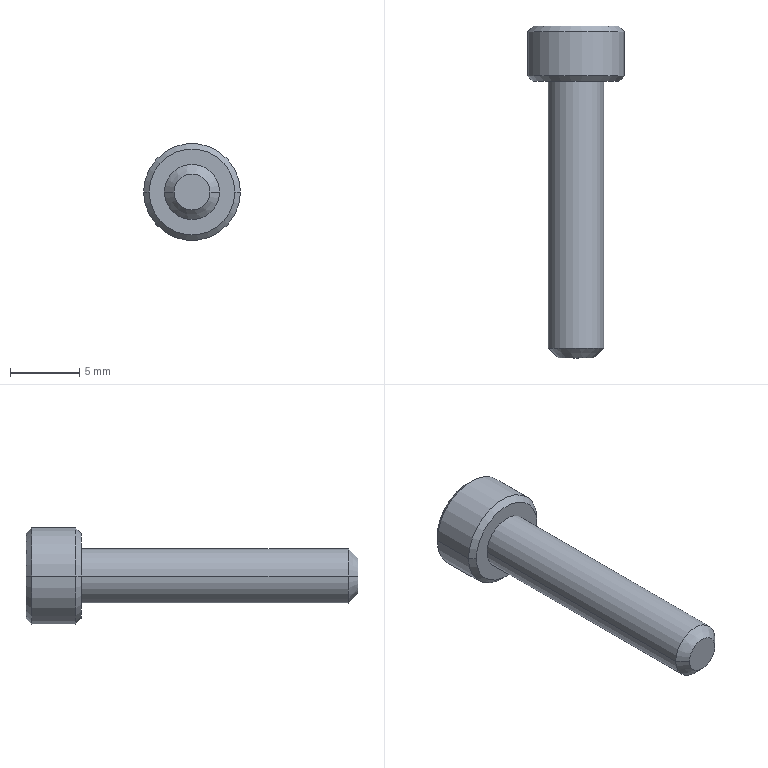Part | STEP file | BB62-M4-20L-3 | 1 solid | 27 faces | box 7 x 24 x 7 mm | volume 380.713 mm3 | plane 15 | cone 8 | cylinder 4 | commonest cylinder face diameters 4 x2 7 x2
STEP:
#1=CARTESIAN_POINT('',(0.,1.007,0.));
#2=VERTEX_POINT('',#1);
#3=CARTESIAN_POINT('',(1.72,2.,0.));
#4=VERTEX_POINT('',#3);
#5=CARTESIAN_POINT('',(0.,1.007,0.));
#6=DIRECTION('',(0.866,0.5,0.));
#7=VECTOR('',#6,1000.);
#8=LINE('',#5,#7);
#9=EDGE_CURVE('',#2,#4,#8,.T.);
#10=ORIENTED_EDGE('',*,*,#9,.F.);
#11=CARTESIAN_POINT('',(-1.72,2.,0.));
#12=VERTEX_POINT('',#11);
#13=CARTESIAN_POINT('',(0.,1.007,0.));
#14=DIRECTION('',(-0.866,0.5,0.));
#15=VECTOR('',#14,1000.);
#16=LINE('',#13,#15);
#17=EDGE_CURVE('',#2,#12,#16,.T.);
#18=ORIENTED_EDGE('',*,*,#17,.T.);
#19=CARTESIAN_POINT('',(-1.49,2.,0.86));
#20=VERTEX_POINT('',#19);
#21=CARTESIAN_POINT('',(0.,2.,0.));
#22=DIRECTION('',(0.,-1.,0.));
#23=DIRECTION('',(-1.,0.,0.));
#24=AXIS2_PLACEMENT_3D('',#21,#22,#23);
#25=CIRCLE('',#24,1.72);
#26=EDGE_CURVE('',#20,#12,#25,.T.);
#27=ORIENTED_EDGE('',*,*,#26,.F.);
#28=CARTESIAN_POINT('',(0.,2.,1.72));
#29=VERTEX_POINT('',#28);
#30=CARTESIAN_POINT('',(0.,2.,0.));
#31=DIRECTION('',(0.,-1.,0.));
#32=DIRECTION('',(-1.,0.,0.));
#33=AXIS2_PLACEMENT_3D('',#30,#31,#32);
#34=CIRCLE('',#33,1.72);
#35=EDGE_CURVE('',#29,#20,#34,.T.);
#36=ORIENTED_EDGE('',*,*,#35,.F.);
#37=CARTESIAN_POINT('',(1.49,2.,0.86));
#38=VERTEX_POINT('',#37);
#39=CARTESIAN_POINT('',(0.,2.,0.));
#40=DIRECTION('',(0.,-1.,0.));
#41=DIRECTION('',(-1.,0.,0.));
#42=AXIS2_PLACEMENT_3D('',#39,#40,#41);
#43=CIRCLE('',#42,1.72);
#44=EDGE_CURVE('',#38,#29,#43,.T.);
#45=ORIENTED_EDGE('',*,*,#44,.F.);
#46=CARTESIAN_POINT('',(0.,2.,0.));
#47=DIRECTION('',(0.,-1.,0.));
#48=DIRECTION('',(-1.,0.,0.));
#49=AXIS2_PLACEMENT_3D('',#46,#47,#48);
#50=CIRCLE('',#49,1.72);
#51=EDGE_CURVE('',#4,#38,#50,.T.);
#52=ORIENTED_EDGE('',*,*,#51,.F.);
#53=EDGE_LOOP('',(#10,#18,#27,#36,#45,#52));
#54=FACE_OUTER_BOUND('',#53,.T.);
#55=CARTESIAN_POINT('',(0.,1001.007,0.));
#56=DIRECTION('',(0.,1.,0.));
#57=DIRECTION('',(1.,0.,0.));
#58=AXIS2_PLACEMENT_3D('',#55,#56,#57);
#59=CONICAL_SURFACE('',#58,1732.051,1.047);
#60=ADVANCED_FACE('',(#54),#59,.F.);
#61=CARTESIAN_POINT('',(1.3,-20.,0.));
#62=VERTEX_POINT('',#61);
#63=CARTESIAN_POINT('',(-1.3,-20.,0.));
#64=VERTEX_POINT('',#63);
#65=CARTESIAN_POINT('',(0.,-20.,0.));
#66=DIRECTION('',(0.,1.,0.));
#67=DIRECTION('',(1.,0.,0.));
#68=AXIS2_PLACEMENT_3D('',#65,#66,#67);
#69=CIRCLE('',#68,1.3);
#70=EDGE_CURVE('',#62,#64,#69,.T.);
#71=ORIENTED_EDGE('',*,*,#70,.T.);
#72=CARTESIAN_POINT('',(-2.,-19.3,0.));
#73=VERTEX_POINT('',#72);
#74=CARTESIAN_POINT('',(-1.3,-20.,0.));
#75=DIRECTION('',(-0.7071,0.7071,0.));
#76=VECTOR('',#75,1000.);
#77=LINE('',#74,#76);
#78=EDGE_CURVE('',#64,#73,#77,.T.);
#79=ORIENTED_EDGE('',*,*,#78,.T.);
#80=CARTESIAN_POINT('',(2.,-19.3,0.));
#81=VERTEX_POINT('',#80);
#82=CARTESIAN_POINT('',(0.,-19.3,0.));
#83=DIRECTION('',(0.,-1.,0.));
#84=DIRECTION('',(-1.,0.,0.));
#85=AXIS2_PLACEMENT_3D('',#82,#83,#84);
#86=CIRCLE('',#85,2.);
#87=EDGE_CURVE('',#73,#81,#86,.T.);
#88=ORIENTED_EDGE('',*,*,#87,.T.);
#89=CARTESIAN_POINT('',(1.3,-20.,0.));
#90=DIRECTION('',(0.7071,0.7071,0.));
#91=VECTOR('',#90,1000.);
#92=LINE('',#89,#91);
#93=EDGE_CURVE('',#62,#81,#92,.T.);
#94=ORIENTED_EDGE('',*,*,#93,.F.);
#95=EDGE_LOOP('',(#71,#79,#88,#94));
#96=FACE_OUTER_BOUND('',#95,.T.);
#97=CARTESIAN_POINT('',(0.,-20.,0.));
#98=DIRECTION('',(0.,1.,0.));
#99=DIRECTION('',(1.,0.,0.));
#100=AXIS2_PLACEMENT_3D('',#97,#98,#99);
#101=CONICAL_SURFACE('',#100,1.3,0.7854);
#102=ADVANCED_FACE('',(#96),#101,.T.);
#103=ORIENTED_EDGE('',*,*,#87,.F.);
#104=CARTESIAN_POINT('',(-2.,0.,0.));
#105=VERTEX_POINT('',#104);
#106=CARTESIAN_POINT('',(-2.,-19.3,0.));
#107=DIRECTION('',(0.,1.,0.));
#108=VECTOR('',#107,1000.);
#109=LINE('',#106,#108);
#110=EDGE_CURVE('',#73,#105,#109,.T.);
#111=ORIENTED_EDGE('',*,*,#110,.T.);
#112=CARTESIAN_POINT('',(2.,0.,0.));
#113=VERTEX_POINT('',#112);
#114=CARTESIAN_POINT('',(0.,0.,0.));
#115=DIRECTION('',(0.,-1.,0.));
#116=DIRECTION('',(-1.,0.,0.));
#117=AXIS2_PLACEMENT_3D('',#114,#115,#116);
#118=CIRCLE('',#117,2.);
#119=EDGE_CURVE('',#105,#113,#118,.T.);
#120=ORIENTED_EDGE('',*,*,#119,.T.);
#121=CARTESIAN_POINT('',(2.,-19.3,0.));
#122=DIRECTION('',(0.,1.,0.));
#123=VECTOR('',#122,1000.);
#124=LINE('',#121,#123);
#125=EDGE_CURVE('',#81,#113,#124,.T.);
#126=ORIENTED_EDGE('',*,*,#125,.F.);
#127=EDGE_LOOP('',(#103,#111,#120,#126));
#128=FACE_OUTER_BOUND('',#127,.T.);
#129=CARTESIAN_POINT('',(0.,-19.3,0.));
#130=DIRECTION('',(0.,1.,0.));
#131=DIRECTION('',(1.,0.,0.));
#132=AXIS2_PLACEMENT_3D('',#129,#130,#131);
#133=CYLINDRICAL_SURFACE('',#132,2.);
#134=ADVANCED_FACE('',(#128),#133,.T.);
#135=CARTESIAN_POINT('',(-3.1,4.,0.));
#136=VERTEX_POINT('',#135);
#137=CARTESIAN_POINT('',(3.1,4.,0.));
#138=VERTEX_POINT('',#137);
#139=CARTESIAN_POINT('',(0.,4.,0.));
#140=DIRECTION('',(0.,-1.,0.));
#141=DIRECTION('',(-1.,0.,0.));
#142=AXIS2_PLACEMENT_3D('',#139,#140,#141);
#143=CIRCLE('',#142,3.1);
#144=EDGE_CURVE('',#136,#138,#143,.T.);
#145=ORIENTED_EDGE('',*,*,#144,.T.);
#146=CARTESIAN_POINT('',(3.5,3.6,0.));
#147=VERTEX_POINT('',#146);
#148=CARTESIAN_POINT('',(3.5,3.6,0.));
#149=DIRECTION('',(0.7071,-0.7071,0.));
#150=VECTOR('',#149,1000.);
#151=LINE('',#148,#150);
#152=EDGE_CURVE('',#138,#147,#151,.T.);
#153=ORIENTED_EDGE('',*,*,#152,.T.);
#154=CARTESIAN_POINT('',(-3.5,3.6,0.));
#155=VERTEX_POINT('',#154);
#156=CARTESIAN_POINT('',(0.,3.6,0.));
#157=DIRECTION('',(0.,-1.,0.));
#158=DIRECTION('',(-1.,0.,0.));
#159=AXIS2_PLACEMENT_3D('',#156,#157,#158);
#160=CIRCLE('',#159,3.5);
#161=EDGE_CURVE('',#155,#147,#160,.T.);
#162=ORIENTED_EDGE('',*,*,#161,.F.);
#163=CARTESIAN_POINT('',(-3.5,3.6,0.));
#164=DIRECTION('',(-0.7071,-0.7071,0.));
#165=VECTOR('',#164,1000.);
#166=LINE('',#163,#165);
#167=EDGE_CURVE('',#136,#155,#166,.T.);
#168=ORIENTED_EDGE('',*,*,#167,.F.);
#169=EDGE_LOOP('',(#145,#153,#162,#168));
#170=FACE_OUTER_BOUND('',#169,.T.);
#171=CARTESIAN_POINT('',(0.,3.6,0.));
#172=DIRECTION('',(0.,-1.,0.));
#173=DIRECTION('',(-1.,0.,0.));
#174=AXIS2_PLACEMENT_3D('',#171,#172,#173);
#175=CONICAL_SURFACE('',#174,3.5,0.7854);
#176=ADVANCED_FACE('',(#170),#175,.T.);
#177=ORIENTED_EDGE('',*,*,#161,.T.);
#178=CARTESIAN_POINT('',(3.5,0.4,0.));
#179=VERTEX_POINT('',#178);
#180=CARTESIAN_POINT('',(3.5,1.62,0.));
#181=DIRECTION('',(0.,-1.,0.));
#182=VECTOR('',#181,1000.);
#183=LINE('',#180,#182);
#184=EDGE_CURVE('',#147,#179,#183,.T.);
#185=ORIENTED_EDGE('',*,*,#184,.T.);
#186=CARTESIAN_POINT('',(-3.5,0.4,0.));
#187=VERTEX_POINT('',#186);
#188=CARTESIAN_POINT('',(0.,0.4,0.));
#189=DIRECTION('',(0.,-1.,0.));
#190=DIRECTION('',(-1.,0.,0.));
#191=AXIS2_PLACEMENT_3D('',#188,#189,#190);
#192=CIRCLE('',#191,3.5);
#193=EDGE_CURVE('',#187,#179,#192,.T.);
#194=ORIENTED_EDGE('',*,*,#193,.F.);
#195=CARTESIAN_POINT('',(-3.5,1.62,0.));
#196=DIRECTION('',(0.,-1.,0.));
#197=VECTOR('',#196,1000.);
#198=LINE('',#195,#197);
#199=EDGE_CURVE('',#155,#187,#198,.T.);
#200=ORIENTED_EDGE('',*,*,#199,.F.);
#201=EDGE_LOOP('',(#177,#185,#194,#200));
#202=FACE_OUTER_BOUND('',#201,.T.);
#203=CARTESIAN_POINT('',(0.,1.62,0.));
#204=DIRECTION('',(0.,-1.,0.));
#205=DIRECTION('',(-1.,0.,0.));
#206=AXIS2_PLACEMENT_3D('',#203,#204,#205);
#207=CYLINDRICAL_SURFACE('',#206,3.5);
#208=ADVANCED_FACE('',(#202),#207,.T.);
#209=CARTESIAN_POINT('',(-3.1,0.,0.));
#210=VERTEX_POINT('',#209);
#211=CARTESIAN_POINT('',(3.1,0.,0.));
#212=VERTEX_POINT('',#211);
#213=CARTESIAN_POINT('',(0.,0.,0.));
#214=DIRECTION('',(0.,-1.,0.));
#215=DIRECTION('',(-1.,0.,0.));
#216=AXIS2_PLACEMENT_3D('',#213,#214,#215);
#217=CIRCLE('',#216,3.1);
#218=EDGE_CURVE('',#210,#212,#217,.T.);
#219=ORIENTED_EDGE('',*,*,#218,.F.);
#220=CARTESIAN_POINT('',(-3.1,0.,0.));
#221=DIRECTION('',(-0.7071,0.7071,0.));
#222=VECTOR('',#221,1000.);
#223=LINE('',#220,#222);
#224=EDGE_CURVE('',#210,#187,#223,.T.);
#225=ORIENTED_EDGE('',*,*,#224,.T.);
#226=ORIENTED_EDGE('',*,*,#193,.T.);
#227=CARTESIAN_POINT('',(3.1,0.,0.));
#228=DIRECTION('',(0.7071,0.7071,0.));
#229=VECTOR('',#228,1000.);
#230=LINE('',#227,#229);
#231=EDGE_CURVE('',#212,#179,#230,.T.);
#232=ORIENTED_EDGE('',*,*,#231,.F.);
#233=EDGE_LOOP('',(#219,#225,#226,#232));
#234=FACE_OUTER_BOUND('',#233,.T.);
#235=CARTESIAN_POINT('',(0.,0.,0.));
#236=DIRECTION('',(0.,1.,0.));
#237=DIRECTION('',(1.,0.,0.));
#238=AXIS2_PLACEMENT_3D('',#235,#236,#237);
#239=CONICAL_SURFACE('',#238,3.1,0.7854);
#240=ADVANCED_FACE('',(#234),#239,.T.);
#241=ORIENTED_EDGE('',*,*,#144,.F.);
#242=CARTESIAN_POINT('',(0.,4.,0.));
#243=DIRECTION('',(0.,-1.,0.));
#244=DIRECTION('',(-1.,0.,0.));
#245=AXIS2_PLACEMENT_3D('',#242,#243,#244);
#246=CIRCLE('',#245,3.1);
#247=EDGE_CURVE('',#138,#136,#246,.T.);
#248=ORIENTED_EDGE('',*,*,#247,.F.);
#249=EDGE_LOOP('',(#241,#248));
#250=FACE_OUTER_BOUND('',#249,.T.);
#251=CARTESIAN_POINT('',(0.,4.,-1.72));
#252=VERTEX_POINT('',#251);
#253=CARTESIAN_POINT('',(-1.49,4.,-0.86));
#254=VERTEX_POINT('',#253);
#255=CARTESIAN_POINT('',(0.,4.,-1.72));
#256=DIRECTION('',(-0.866,0.,0.5));
#257=VECTOR('',#256,1000.);
#258=LINE('',#255,#257);
#259=EDGE_CURVE('',#252,#254,#258,.T.);
#260=ORIENTED_EDGE('',*,*,#259,.F.);
#261=CARTESIAN_POINT('',(1.49,4.,-0.86));
#262=VERTEX_POINT('',#261);
#263=CARTESIAN_POINT('',(1.49,4.,-0.86));
#264=DIRECTION('',(-0.866,0.,-0.5));
#265=VECTOR('',#264,1000.);
#266=LINE('',#263,#265);
#267=EDGE_CURVE('',#262,#252,#266,.T.);
#268=ORIENTED_EDGE('',*,*,#267,.F.);
#269=CARTESIAN_POINT('',(1.49,4.,0.86));
#270=VERTEX_POINT('',#269);
#271=CARTESIAN_POINT('',(1.49,4.,0.86));
#272=DIRECTION('',(0.,0.,-1.));
#273=VECTOR('',#272,1000.);
#274=LINE('',#271,#273);
#275=EDGE_CURVE('',#270,#262,#274,.T.);
#276=ORIENTED_EDGE('',*,*,#275,.F.);
#277=CARTESIAN_POINT('',(0.,4.,1.72));
#278=VERTEX_POINT('',#277);
#279=CARTESIAN_POINT('',(0.,4.,1.72));
#280=DIRECTION('',(0.866,0.,-0.5));
#281=VECTOR('',#280,1000.);
#282=LINE('',#279,#281);
#283=EDGE_CURVE('',#278,#270,#282,.T.);
#284=ORIENTED_EDGE('',*,*,#283,.F.);
#285=CARTESIAN_POINT('',(-1.49,4.,0.86));
#286=VERTEX_POINT('',#285);
#287=CARTESIAN_POINT('',(-1.49,4.,0.86));
#288=DIRECTION('',(0.866,0.,0.5));
#289=VECTOR('',#288,1000.);
#290=LINE('',#287,#289);
#291=EDGE_CURVE('',#286,#278,#290,.T.);
#292=ORIENTED_EDGE('',*,*,#291,.F.);
#293=CARTESIAN_POINT('',(-1.49,4.,-0.86));
#294=DIRECTION('',(0.,0.,1.));
#295=VECTOR('',#294,1000.);
#296=LINE('',#293,#295);
#297=EDGE_CURVE('',#254,#286,#296,.T.);
#298=ORIENTED_EDGE('',*,*,#297,.F.);
#299=EDGE_LOOP('',(#260,#268,#276,#284,#292,#298));
#300=FACE_BOUND('',#299,.T.);
#301=CARTESIAN_POINT('',(3.1,4.,0.));
#302=DIRECTION('',(0.,1.,0.));
#303=DIRECTION('',(1.,0.,0.));
#304=AXIS2_PLACEMENT_3D('',#301,#302,#303);
#305=PLANE('',#304);
#306=ADVANCED_FACE('',(#250,#300),#305,.T.);
#307=CARTESIAN_POINT('',(0.,0.,0.));
#308=DIRECTION('',(0.,-1.,0.));
#309=DIRECTION('',(-1.,0.,0.));
#310=AXIS2_PLACEMENT_3D('',#307,#308,#309);
#311=CIRCLE('',#310,2.);
#312=EDGE_CURVE('',#113,#105,#311,.T.);
#313=ORIENTED_EDGE('',*,*,#312,.F.);
#314=ORIENTED_EDGE('',*,*,#119,.F.);
#315=EDGE_LOOP('',(#313,#314));
#316=FACE_BOUND('',#315,.T.);
#317=CARTESIAN_POINT('',(0.,0.,0.));
#318=DIRECTION('',(0.,-1.,0.));
#319=DIRECTION('',(-1.,0.,0.));
#320=AXIS2_PLACEMENT_3D('',#317,#318,#319);
#321=CIRCLE('',#320,3.1);
#322=EDGE_CURVE('',#212,#210,#321,.T.);
#323=ORIENTED_EDGE('',*,*,#322,.T.);
#324=ORIENTED_EDGE('',*,*,#218,.T.);
#325=EDGE_LOOP('',(#323,#324));
#326=FACE_OUTER_BOUND('',#325,.T.);
#327=CARTESIAN_POINT('',(0.,0.,0.));
#328=DIRECTION('',(0.,-1.,0.));
#329=DIRECTION('',(-1.,0.,0.));
#330=AXIS2_PLACEMENT_3D('',#327,#328,#329);
#331=PLANE('',#330);
#332=ADVANCED_FACE('',(#316,#326),#331,.T.);
#333=ORIENTED_EDGE('',*,*,#224,.F.);
#334=ORIENTED_EDGE('',*,*,#322,.F.);
#335=ORIENTED_EDGE('',*,*,#231,.T.);
#336=CARTESIAN_POINT('',(0.,0.4,0.));
#337=DIRECTION('',(0.,-1.,0.));
#338=DIRECTION('',(-1.,0.,0.));
#339=AXIS2_PLACEMENT_3D('',#336,#337,#338);
#340=CIRCLE('',#339,3.5);
#341=EDGE_CURVE('',#179,#187,#340,.T.);
#342=ORIENTED_EDGE('',*,*,#341,.T.);
#343=EDGE_LOOP('',(#333,#334,#335,#342));
#344=FACE_OUTER_BOUND('',#343,.T.);
#345=CARTESIAN_POINT('',(0.,0.,0.));
#346=DIRECTION('',(0.,1.,0.));
#347=DIRECTION('',(1.,0.,0.));
#348=AXIS2_PLACEMENT_3D('',#345,#346,#347);
#349=CONICAL_SURFACE('',#348,3.1,0.7854);
#350=ADVANCED_FACE('',(#344),#349,.T.);
#351=ORIENTED_EDGE('',*,*,#184,.F.);
#352=CARTESIAN_POINT('',(0.,3.6,0.));
#353=DIRECTION('',(0.,-1.,0.));
#354=DIRECTION('',(-1.,0.,0.));
#355=AXIS2_PLACEMENT_3D('',#352,#353,#354);
#356=CIRCLE('',#355,3.5);
#357=EDGE_CURVE('',#147,#155,#356,.T.);
#358=ORIENTED_EDGE('',*,*,#357,.T.);
#359=ORIENTED_EDGE('',*,*,#199,.T.);
#360=ORIENTED_EDGE('',*,*,#341,.F.);
#361=EDGE_LOOP('',(#351,#358,#359,#360));
#362=FACE_OUTER_BOUND('',#361,.T.);
#363=CARTESIAN_POINT('',(0.,1.62,0.));
#364=DIRECTION('',(0.,-1.,0.));
#365=DIRECTION('',(-1.,0.,0.));
#366=AXIS2_PLACEMENT_3D('',#363,#364,#365);
#367=CYLINDRICAL_SURFACE('',#366,3.5);
#368=ADVANCED_FACE('',(#362),#367,.T.);
#369=ORIENTED_EDGE('',*,*,#152,.F.);
#370=ORIENTED_EDGE('',*,*,#247,.T.);
#371=ORIENTED_EDGE('',*,*,#167,.T.);
#372=ORIENTED_EDGE('',*,*,#357,.F.);
#373=EDGE_LOOP('',(#369,#370,#371,#372));
#374=FACE_OUTER_BOUND('',#373,.T.);
#375=CARTESIAN_POINT('',(0.,3.6,0.));
#376=DIRECTION('',(0.,-1.,0.));
#377=DIRECTION('',(-1.,0.,0.));
#378=AXIS2_PLACEMENT_3D('',#375,#376,#377);
#379=CONICAL_SURFACE('',#378,3.5,0.7854);
#380=ADVANCED_FACE('',(#374),#379,.T.);
#381=ORIENTED_EDGE('',*,*,#110,.F.);
#382=CARTESIAN_POINT('',(0.,-19.3,0.));
#383=DIRECTION('',(0.,-1.,0.));
#384=DIRECTION('',(-1.,0.,0.));
#385=AXIS2_PLACEMENT_3D('',#382,#383,#384);
#386=CIRCLE('',#385,2.);
#387=EDGE_CURVE('',#81,#73,#386,.T.);
#388=ORIENTED_EDGE('',*,*,#387,.F.);
#389=ORIENTED_EDGE('',*,*,#125,.T.);
#390=ORIENTED_EDGE('',*,*,#312,.T.);
#391=EDGE_LOOP('',(#381,#388,#389,#390));
#392=FACE_OUTER_BOUND('',#391,.T.);
#393=CARTESIAN_POINT('',(0.,-19.3,0.));
#394=DIRECTION('',(0.,1.,0.));
#395=DIRECTION('',(1.,0.,0.));
#396=AXIS2_PLACEMENT_3D('',#393,#394,#395);
#397=CYLINDRICAL_SURFACE('',#396,2.);
#398=ADVANCED_FACE('',(#392),#397,.T.);
#399=ORIENTED_EDGE('',*,*,#70,.F.);
#400=CARTESIAN_POINT('',(0.,-20.,0.));
#401=DIRECTION('',(0.,1.,0.));
#402=DIRECTION('',(1.,0.,0.));
#403=AXIS2_PLACEMENT_3D('',#400,#401,#402);
#404=CIRCLE('',#403,1.3);
#405=EDGE_CURVE('',#64,#62,#404,.T.);
#406=ORIENTED_EDGE('',*,*,#405,.F.);
#407=EDGE_LOOP('',(#399,#406));
#408=FACE_OUTER_BOUND('',#407,.T.);
#409=CARTESIAN_POINT('',(0.,-20.,0.));
#410=DIRECTION('',(0.,-1.,0.));
#411=DIRECTION('',(-1.,0.,0.));
#412=AXIS2_PLACEMENT_3D('',#409,#410,#411);
#413=PLANE('',#412);
#414=ADVANCED_FACE('',(#408),#413,.T.);
#415=ORIENTED_EDGE('',*,*,#78,.F.);
#416=ORIENTED_EDGE('',*,*,#405,.T.);
#417=ORIENTED_EDGE('',*,*,#93,.T.);
#418=ORIENTED_EDGE('',*,*,#387,.T.);
#419=EDGE_LOOP('',(#415,#416,#417,#418));
#420=FACE_OUTER_BOUND('',#419,.T.);
#421=CARTESIAN_POINT('',(0.,-20.,0.));
#422=DIRECTION('',(0.,1.,0.));
#423=DIRECTION('',(1.,0.,0.));
#424=AXIS2_PLACEMENT_3D('',#421,#422,#423);
#425=CONICAL_SURFACE('',#424,1.3,0.7854);
#426=ADVANCED_FACE('',(#420),#425,.T.);
#427=CARTESIAN_POINT('',(1.49,2.,-0.86));
#428=VERTEX_POINT('',#427);
#429=CARTESIAN_POINT('',(0.,2.,-1.72));
#430=VERTEX_POINT('',#429);
#431=CARTESIAN_POINT('',(1.49,2.,-0.86));
#432=DIRECTION('',(-0.866,0.,-0.5));
#433=VECTOR('',#432,1000.);
#434=LINE('',#431,#433);
#435=EDGE_CURVE('',#428,#430,#434,.T.);
#436=ORIENTED_EDGE('',*,*,#435,.F.);
#437=CARTESIAN_POINT('',(1.49,4.,-0.86));
#438=DIRECTION('',(0.,-1.,0.));
#439=VECTOR('',#438,1000.);
#440=LINE('',#437,#439);
#441=EDGE_CURVE('',#262,#428,#440,.T.);
#442=ORIENTED_EDGE('',*,*,#441,.F.);
#443=ORIENTED_EDGE('',*,*,#267,.T.);
#444=CARTESIAN_POINT('',(0.,4.,-1.72));
#445=DIRECTION('',(0.,-1.,0.));
#446=VECTOR('',#445,1000.);
#447=LINE('',#444,#446);
#448=EDGE_CURVE('',#252,#430,#447,.T.);
#449=ORIENTED_EDGE('',*,*,#448,.T.);
#450=EDGE_LOOP('',(#436,#442,#443,#449));
#451=FACE_OUTER_BOUND('',#450,.T.);
#452=CARTESIAN_POINT('',(1.49,4.,-0.86));
#453=DIRECTION('',(-0.5,0.,0.866));
#454=DIRECTION('',(0.866,0.,0.5));
#455=AXIS2_PLACEMENT_3D('',#452,#453,#454);
#456=PLANE('',#455);
#457=ADVANCED_FACE('',(#451),#456,.T.);
#458=CARTESIAN_POINT('',(-1.49,2.,-0.86));
#459=VERTEX_POINT('',#458);
#460=CARTESIAN_POINT('',(0.,2.,-1.72));
#461=DIRECTION('',(-0.866,0.,0.5));
#462=VECTOR('',#461,1000.);
#463=LINE('',#460,#462);
#464=EDGE_CURVE('',#430,#459,#463,.T.);
#465=ORIENTED_EDGE('',*,*,#464,.F.);
#466=ORIENTED_EDGE('',*,*,#448,.F.);
#467=ORIENTED_EDGE('',*,*,#259,.T.);
#468=CARTESIAN_POINT('',(-1.49,4.,-0.86));
#469=DIRECTION('',(0.,-1.,0.));
#470=VECTOR('',#469,1000.);
#471=LINE('',#468,#470);
#472=EDGE_CURVE('',#254,#459,#471,.T.);
#473=ORIENTED_EDGE('',*,*,#472,.T.);
#474=EDGE_LOOP('',(#465,#466,#467,#473));
#475=FACE_OUTER_BOUND('',#474,.T.);
#476=CARTESIAN_POINT('',(0.,4.,-1.72));
#477=DIRECTION('',(0.5,0.,0.866));
#478=DIRECTION('',(0.866,0.,-0.5));
#479=AXIS2_PLACEMENT_3D('',#476,#477,#478);
#480=PLANE('',#479);
#481=ADVANCED_FACE('',(#475),#480,.T.);
#482=CARTESIAN_POINT('',(-1.49,2.,-0.86));
#483=DIRECTION('',(0.,0.,1.));
#484=VECTOR('',#483,1000.);
#485=LINE('',#482,#484);
#486=EDGE_CURVE('',#459,#20,#485,.T.);
#487=ORIENTED_EDGE('',*,*,#486,.F.);
#488=ORIENTED_EDGE('',*,*,#472,.F.);
#489=ORIENTED_EDGE('',*,*,#297,.T.);
#490=CARTESIAN_POINT('',(-1.49,4.,0.86));
#491=DIRECTION('',(0.,-1.,0.));
#492=VECTOR('',#491,1000.);
#493=LINE('',#490,#492);
#494=EDGE_CURVE('',#286,#20,#493,.T.);
#495=ORIENTED_EDGE('',*,*,#494,.T.);
#496=EDGE_LOOP('',(#487,#488,#489,#495));
#497=FACE_OUTER_BOUND('',#496,.T.);
#498=CARTESIAN_POINT('',(-1.49,4.,-0.86));
#499=DIRECTION('',(1.,0.,0.));
#500=DIRECTION('',(0.,0.,-1.));
#501=AXIS2_PLACEMENT_3D('',#498,#499,#500);
#502=PLANE('',#501);
#503=ADVANCED_FACE('',(#497),#502,.T.);
#504=CARTESIAN_POINT('',(-1.49,2.,0.86));
#505=DIRECTION('',(0.866,0.,0.5));
#506=VECTOR('',#505,1000.);
#507=LINE('',#504,#506);
#508=EDGE_CURVE('',#20,#29,#507,.T.);
#509=ORIENTED_EDGE('',*,*,#508,.F.);
#510=ORIENTED_EDGE('',*,*,#494,.F.);
#511=ORIENTED_EDGE('',*,*,#291,.T.);
#512=CARTESIAN_POINT('',(0.,4.,1.72));
#513=DIRECTION('',(0.,-1.,0.));
#514=VECTOR('',#513,1000.);
#515=LINE('',#512,#514);
#516=EDGE_CURVE('',#278,#29,#515,.T.);
#517=ORIENTED_EDGE('',*,*,#516,.T.);
#518=EDGE_LOOP('',(#509,#510,#511,#517));
#519=FACE_OUTER_BOUND('',#518,.T.);
#520=CARTESIAN_POINT('',(-1.49,4.,0.86));
#521=DIRECTION('',(0.5,0.,-0.866));
#522=DIRECTION('',(-0.866,0.,-0.5));
#523=AXIS2_PLACEMENT_3D('',#520,#521,#522);
#524=PLANE('',#523);
#525=ADVANCED_FACE('',(#519),#524,.T.);
#526=CARTESIAN_POINT('',(0.,2.,1.72));
#527=DIRECTION('',(0.866,0.,-0.5));
#528=VECTOR('',#527,1000.);
#529=LINE('',#526,#528);
#530=EDGE_CURVE('',#29,#38,#529,.T.);
#531=ORIENTED_EDGE('',*,*,#530,.F.);
#532=ORIENTED_EDGE('',*,*,#516,.F.);
#533=ORIENTED_EDGE('',*,*,#283,.T.);
#534=CARTESIAN_POINT('',(1.49,4.,0.86));
#535=DIRECTION('',(0.,-1.,0.));
#536=VECTOR('',#535,1000.);
#537=LINE('',#534,#536);
#538=EDGE_CURVE('',#270,#38,#537,.T.);
#539=ORIENTED_EDGE('',*,*,#538,.T.);
#540=EDGE_LOOP('',(#531,#532,#533,#539));
#541=FACE_OUTER_BOUND('',#540,.T.);
#542=CARTESIAN_POINT('',(0.,4.,1.72));
#543=DIRECTION('',(-0.5,0.,-0.866));
#544=DIRECTION('',(-0.866,0.,0.5));
#545=AXIS2_PLACEMENT_3D('',#542,#543,#544);
#546=PLANE('',#545);
#547=ADVANCED_FACE('',(#541),#546,.T.);
#548=CARTESIAN_POINT('',(1.49,2.,0.86));
#549=DIRECTION('',(0.,0.,-1.));
#550=VECTOR('',#549,1000.);
#551=LINE('',#548,#550);
#552=EDGE_CURVE('',#38,#428,#551,.T.);
#553=ORIENTED_EDGE('',*,*,#552,.F.);
#554=ORIENTED_EDGE('',*,*,#538,.F.);
#555=ORIENTED_EDGE('',*,*,#275,.T.);
#556=ORIENTED_EDGE('',*,*,#441,.T.);
#557=EDGE_LOOP('',(#553,#554,#555,#556));
#558=FACE_OUTER_BOUND('',#557,.T.);
#559=CARTESIAN_POINT('',(1.49,4.,0.86));
#560=DIRECTION('',(-1.,0.,0.));
#561=DIRECTION('',(0.,0.,1.));
#562=AXIS2_PLACEMENT_3D('',#559,#560,#561);
#563=PLANE('',#562);
#564=ADVANCED_FACE('',(#558),#563,.T.);
#565=ORIENTED_EDGE('',*,*,#435,.T.);
#566=CARTESIAN_POINT('',(0.,2.,0.));
#567=DIRECTION('',(0.,-1.,0.));
#568=DIRECTION('',(-1.,0.,0.));
#569=AXIS2_PLACEMENT_3D('',#566,#567,#568);
#570=CIRCLE('',#569,1.72);
#571=EDGE_CURVE('',#430,#428,#570,.T.);
#572=ORIENTED_EDGE('',*,*,#571,.T.);
#573=EDGE_LOOP('',(#565,#572));
#574=FACE_OUTER_BOUND('',#573,.T.);
#575=CARTESIAN_POINT('',(0.,2.,0.));
#576=DIRECTION('',(0.,1.,0.));
#577=DIRECTION('',(1.,0.,0.));
#578=AXIS2_PLACEMENT_3D('',#575,#576,#577);
#579=PLANE('',#578);
#580=ADVANCED_FACE('',(#574),#579,.F.);
#581=ORIENTED_EDGE('',*,*,#552,.T.);
#582=CARTESIAN_POINT('',(0.,2.,0.));
#583=DIRECTION('',(0.,-1.,0.));
#584=DIRECTION('',(-1.,0.,0.));
#585=AXIS2_PLACEMENT_3D('',#582,#583,#584);
#586=CIRCLE('',#585,1.72);
#587=EDGE_CURVE('',#428,#4,#586,.T.);
#588=ORIENTED_EDGE('',*,*,#587,.T.);
#589=ORIENTED_EDGE('',*,*,#51,.T.);
#590=EDGE_LOOP('',(#581,#588,#589));
#591=FACE_OUTER_BOUND('',#590,.T.);
#592=CARTESIAN_POINT('',(0.,2.,0.));
#593=DIRECTION('',(0.,1.,0.));
#594=DIRECTION('',(1.,0.,0.));
#595=AXIS2_PLACEMENT_3D('',#592,#593,#594);
#596=PLANE('',#595);
#597=ADVANCED_FACE('',(#591),#596,.F.);
#598=ORIENTED_EDGE('',*,*,#530,.T.);
#599=ORIENTED_EDGE('',*,*,#44,.T.);
#600=EDGE_LOOP('',(#598,#599));
#601=FACE_OUTER_BOUND('',#600,.T.);
#602=CARTESIAN_POINT('',(0.,2.,0.));
#603=DIRECTION('',(0.,1.,0.));
#604=DIRECTION('',(1.,0.,0.));
#605=AXIS2_PLACEMENT_3D('',#602,#603,#604);
#606=PLANE('',#605);
#607=ADVANCED_FACE('',(#601),#606,.F.);
#608=ORIENTED_EDGE('',*,*,#508,.T.);
#609=ORIENTED_EDGE('',*,*,#35,.T.);
#610=EDGE_LOOP('',(#608,#609));
#611=FACE_OUTER_BOUND('',#610,.T.);
#612=CARTESIAN_POINT('',(0.,2.,0.));
#613=DIRECTION('',(0.,1.,0.));
#614=DIRECTION('',(1.,0.,0.));
#615=AXIS2_PLACEMENT_3D('',#612,#613,#614);
#616=PLANE('',#615);
#617=ADVANCED_FACE('',(#611),#616,.F.);
#618=ORIENTED_EDGE('',*,*,#486,.T.);
#619=ORIENTED_EDGE('',*,*,#26,.T.);
#620=CARTESIAN_POINT('',(0.,2.,0.));
#621=DIRECTION('',(0.,-1.,0.));
#622=DIRECTION('',(-1.,0.,0.));
#623=AXIS2_PLACEMENT_3D('',#620,#621,#622);
#624=CIRCLE('',#623,1.72);
#625=EDGE_CURVE('',#12,#459,#624,.T.);
#626=ORIENTED_EDGE('',*,*,#625,.T.);
#627=EDGE_LOOP('',(#618,#619,#626));
#628=FACE_OUTER_BOUND('',#627,.T.);
#629=CARTESIAN_POINT('',(0.,2.,0.));
#630=DIRECTION('',(0.,1.,0.));
#631=DIRECTION('',(1.,0.,0.));
#632=AXIS2_PLACEMENT_3D('',#629,#630,#631);
#633=PLANE('',#632);
#634=ADVANCED_FACE('',(#628),#633,.F.);
#635=ORIENTED_EDGE('',*,*,#464,.T.);
#636=CARTESIAN_POINT('',(0.,2.,0.));
#637=DIRECTION('',(0.,-1.,0.));
#638=DIRECTION('',(-1.,0.,0.));
#639=AXIS2_PLACEMENT_3D('',#636,#637,#638);
#640=CIRCLE('',#639,1.72);
#641=EDGE_CURVE('',#459,#430,#640,.T.);
#642=ORIENTED_EDGE('',*,*,#641,.T.);
#643=EDGE_LOOP('',(#635,#642));
#644=FACE_OUTER_BOUND('',#643,.T.);
#645=CARTESIAN_POINT('',(0.,2.,0.));
#646=DIRECTION('',(0.,1.,0.));
#647=DIRECTION('',(1.,0.,0.));
#648=AXIS2_PLACEMENT_3D('',#645,#646,#647);
#649=PLANE('',#648);
#650=ADVANCED_FACE('',(#644),#649,.F.);
#651=ORIENTED_EDGE('',*,*,#17,.F.);
#652=ORIENTED_EDGE('',*,*,#9,.T.);
#653=ORIENTED_EDGE('',*,*,#587,.F.);
#654=ORIENTED_EDGE('',*,*,#571,.F.);
#655=ORIENTED_EDGE('',*,*,#641,.F.);
#656=ORIENTED_EDGE('',*,*,#625,.F.);
#657=EDGE_LOOP('',(#651,#652,#653,#654,#655,#656));
#658=FACE_OUTER_BOUND('',#657,.T.);
#659=CARTESIAN_POINT('',(0.,1001.007,0.));
#660=DIRECTION('',(0.,1.,0.));
#661=DIRECTION('',(1.,0.,0.));
#662=AXIS2_PLACEMENT_3D('',#659,#660,#661);
#663=CONICAL_SURFACE('',#662,1732.051,1.047);
#664=ADVANCED_FACE('',(#658),#663,.F.);
#665=CLOSED_SHELL('',(#60,#102,#134,#176,#208,#240,#306,#332,#350,#368,#380,#398,#414,#426,#457,#481,#503,#525,#547,#564,#580,#597,#607,#617,#634,#650,#664));
#666=MANIFOLD_SOLID_BREP('',#665);
#667=CARTESIAN_POINT('',(0.,0.,0.));
#668=DIRECTION('',(0.,0.,1.));
#669=DIRECTION('',(1.,0.,0.));
#670=AXIS2_PLACEMENT_3D('',#667,#668,#669);
#671=(LENGTH_UNIT()NAMED_UNIT(*)SI_UNIT(.MILLI.,.METRE.));
#672=UNCERTAINTY_MEASURE_WITH_UNIT(LENGTH_MEASURE(0.00001),#671,'','');
#673=(NAMED_UNIT(*)PLANE_ANGLE_UNIT()SI_UNIT($,.RADIAN.));
#674=(NAMED_UNIT(*)SI_UNIT($,.STERADIAN.)SOLID_ANGLE_UNIT());
#675=(GEOMETRIC_REPRESENTATION_CONTEXT(3)GLOBAL_UNCERTAINTY_ASSIGNED_CONTEXT((#672))GLOBAL_UNIT_ASSIGNED_CONTEXT((#671,#673,#674))REPRESENTATION_CONTEXT('',''));
#676=ADVANCED_BREP_SHAPE_REPRESENTATION('',(#666,#670),#675);